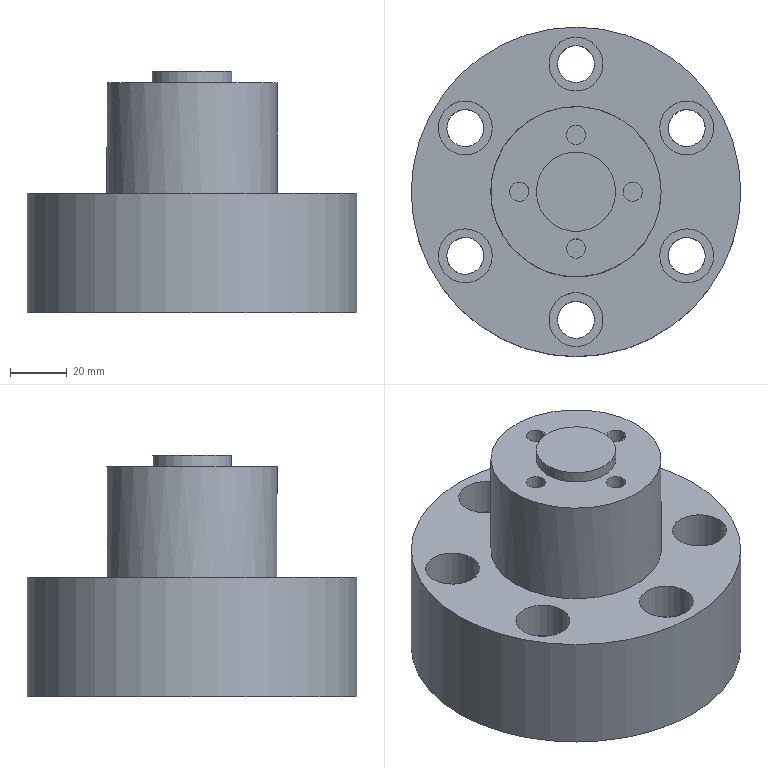NC program | NX | posted with a generic post | part box 116 x 116 x 85 mm
Whole program:
N10 G17 G21 G94 G90
(DRILLING , TOOL : ZXZ)
N12 T01 M6
N14 G54
N16 G17 G0 G90 X38.971 Y-22.5 S3000 M3
N18 G43 Z30. H1
N20 G94 G81 G98 Z-44. F250. R-40.
N22 Y22.5
N24 X0. Y45.
N26 X-38.971 Y22.5
N28 Y-22.5
N30 X0. Y-45.
N32 Y-20. Z-5. R-1.
N34 X-20. Y0.
N36 X0. Y20.
N38 X20. Y0.
N40 G80
N42 G0 X20. Y0. Z30.
N44 M5
(DRILLING_COPY , TOOL : 6.8ZT)
N46 T02 M6
N48 G54
N50 G17 G0 G90 X0. Y20. S2000 M3
N52 G43 Z30. H2
N54 G94 G83 G98 Z-22.043 F150. Q2. R-1.
N56 X-20. Y0.
N58 X0. Y-20.
N60 X20. Y0.
N62 G80
N64 G0 X20. Y0. Z30.
N66 M5
(DRILLING_COPY_COPY , TOOL : 13.0ZT)
N68 T03 M6
N70 G54
N72 G17 G0 G90 X0. Y-45. S600 M3
N74 G43 Z30. H3
N76 G94 G83 G98 Z-90.406 F150. Q4. R-40.
N78 X38.971 Y-22.5
N80 Y22.5
N82 X0. Y45.
N84 X-38.971 Y22.5
N86 Y-22.5
N88 G80
N90 G0 X-38.971 Y-22.5 Z30.
N92 M5
N94 M2